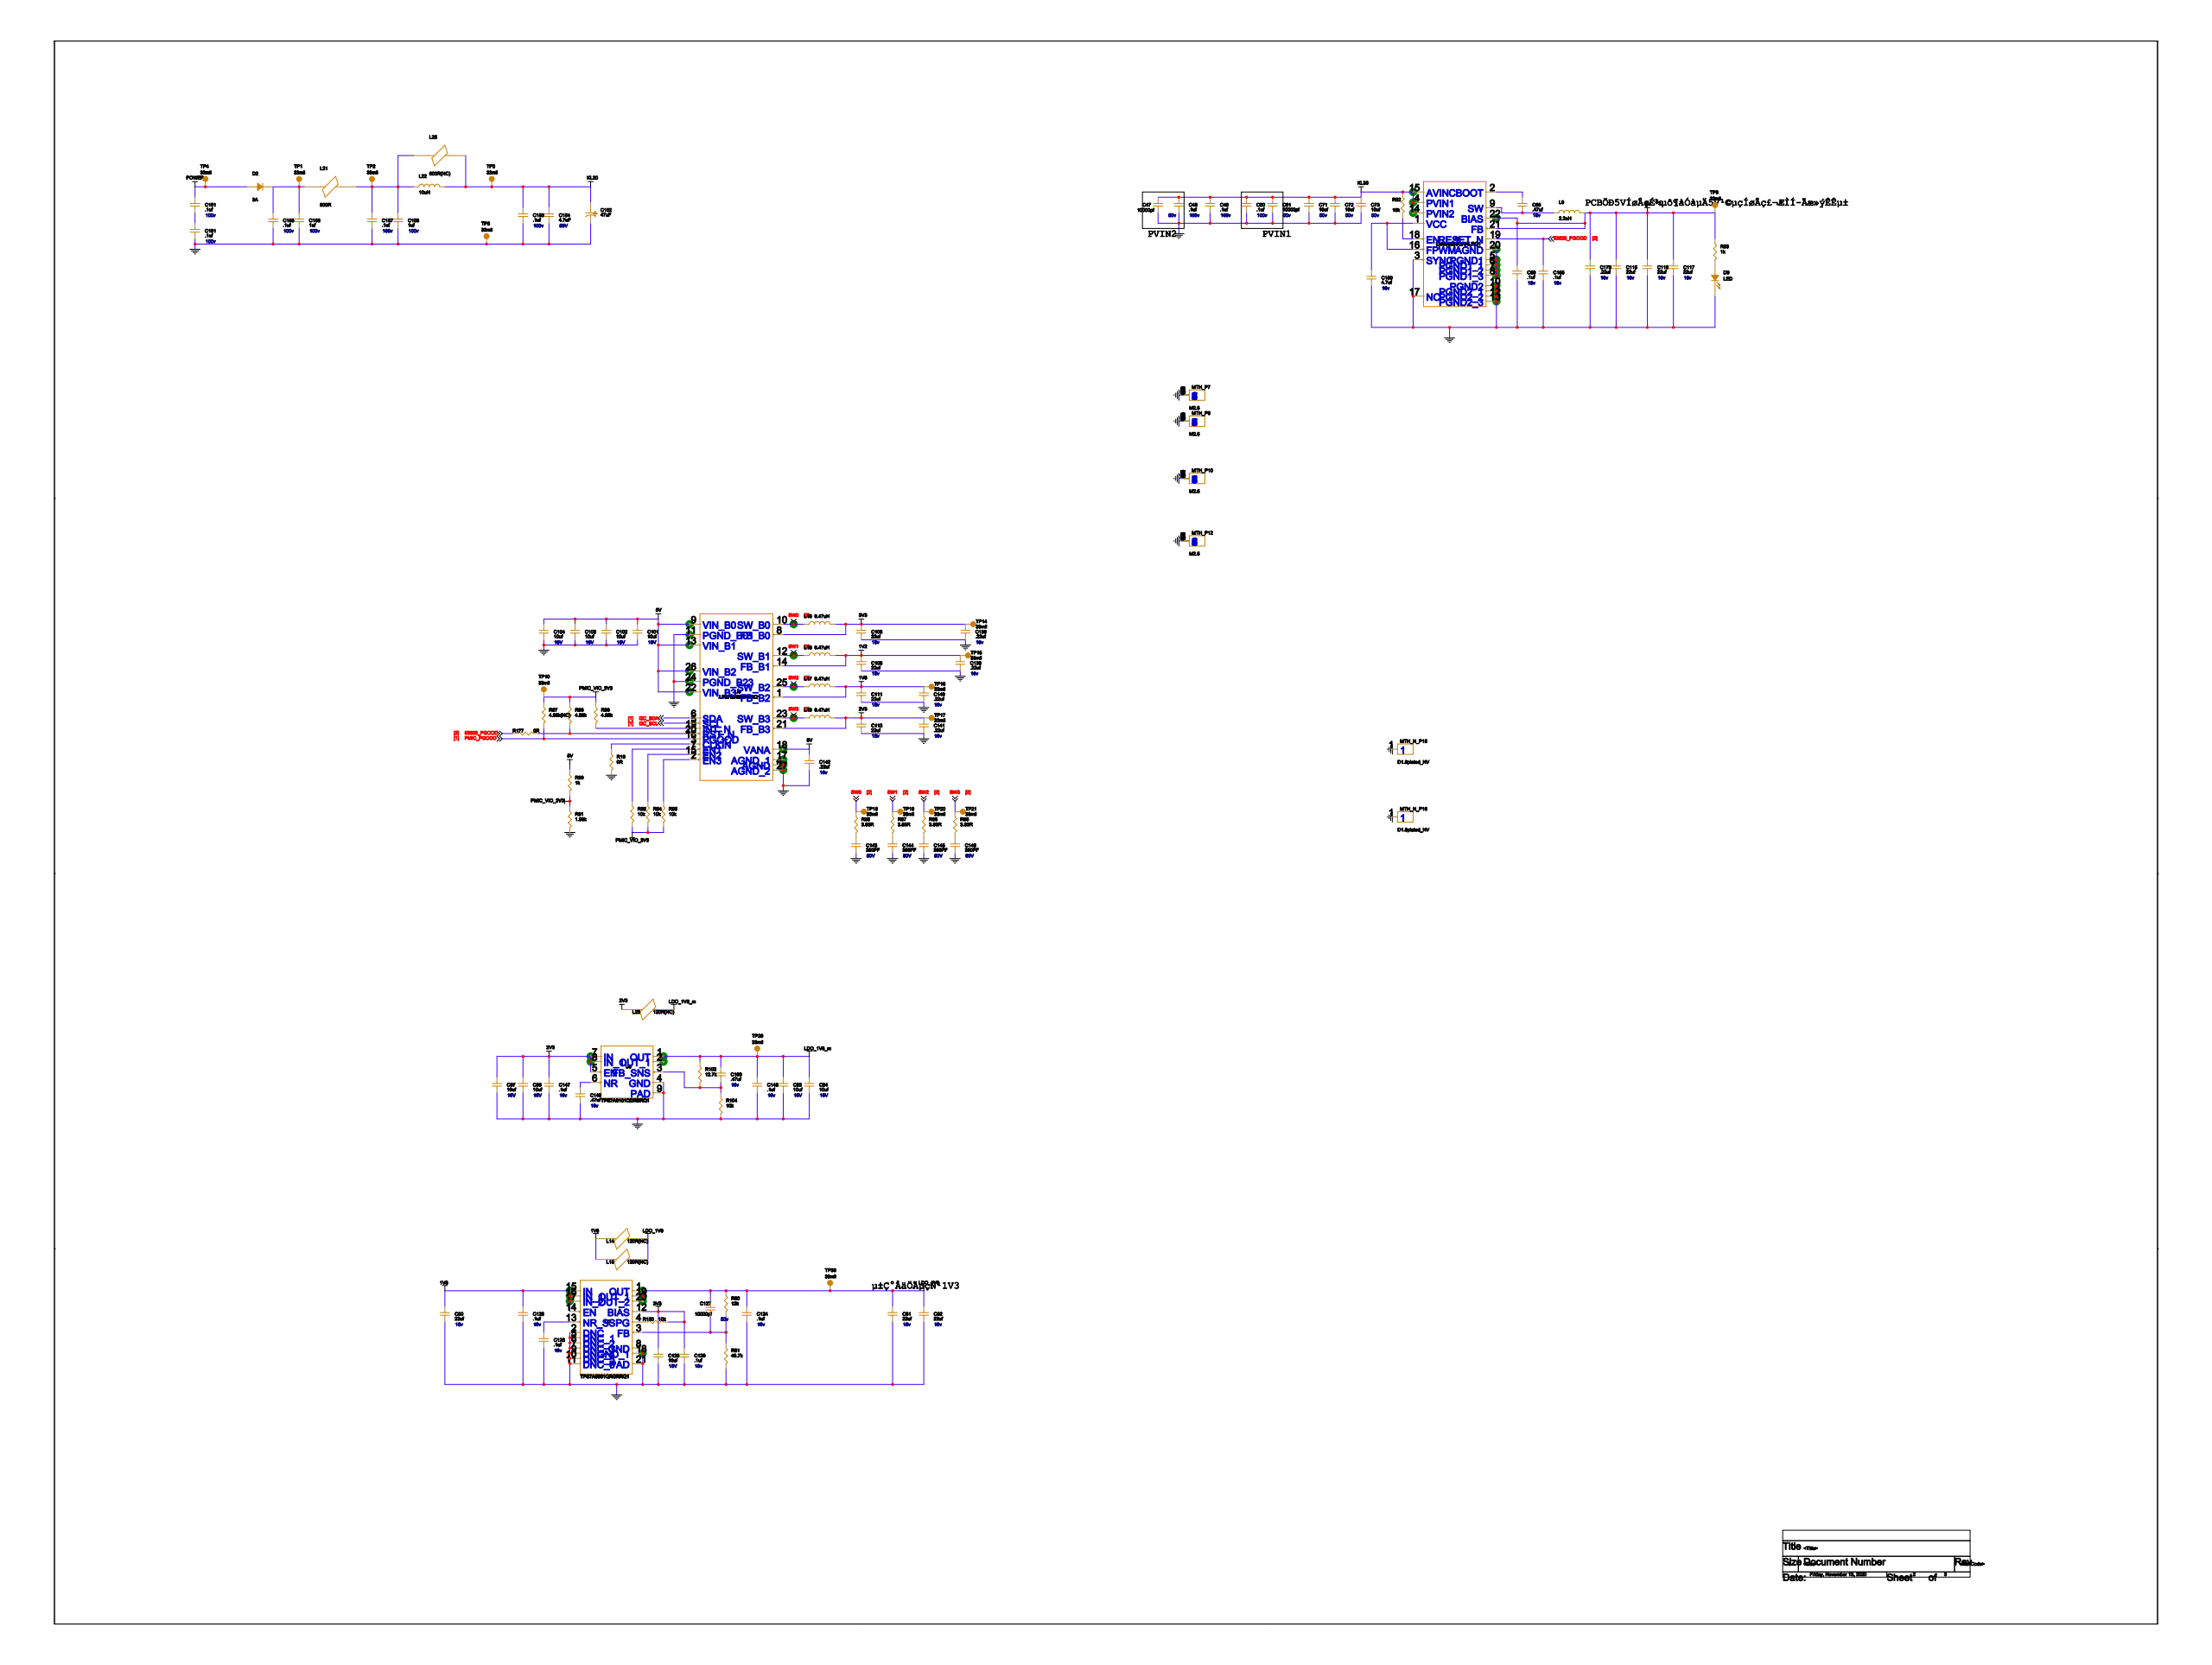Circuit board | Cadence Allegro | 338 parts | 150 nets | one sheet of the schematic
Parts on this sheet (reference | value | footprint):
C47 | 10000pf | C0402
C48 | .1uf | C0805
C49 | .1uf | C0805
C50 | .1uf | C0805
C51 | 10000pf | C0402
C55 | .47uf | C0603
C59 | .1uf | C0402
C71 | 10uf | C1210
C72 | 10uf | C1210
C73 | 10uf | C1210
C80 | 22uf | C1210
C81 | 22uf | C1210
C82 | 22uf | C1210
C83 | 10uf | C0805
C84 | 10uf | C0805
C86 | 10uf | C0805
C87 | 10uf | C0805
C101 | 10uf | C0805
C102 | 10uf | C0805
C103 | 10uf | C0805
C104 | 10uf | C0805
C105 | 22uf | C1210
C108 | 22uf | C1210
C111 | 22uf | C1210
C113 | 22uf | C1210
C115 | 22uf | C1210
C116 | 22uf | C1210
C117 | 22uf | C1210
C124 | .1uf | C0402
C125 | .1uf | C0402
C126 | .1uf | C0402
C127 | 10000pf | C0402
C128 | 10uf | C0805
C129 | .1uf | C0402
C138 | .22uf | C0402
C139 | .22uf | C0402
C140 | .22uf | C0402
C141 | .22uf | C0402
C142 | .22uf | C0402
C143 | 390PF | C0402
C144 | 390PF | C0402
C145 | 390PF | C0402
C146 | 390PF | C0402
C147 | .1uf | C0402
C148 | .1uf | C0402
C149 | .47uf | C0603
C151 | .1uf | C0805
C152 | 47uF | CAPAE630X800N
C153 | .1uf | C0805
C154 | 4.7uF | C0805
C155 | .1uf | C0805
C156 | 1uf | C0805
C157 | .1uf | C0805
C158 | 1uf | C0805
C161 | .1uf | C0805
C163 | .47uf | C0603
C179 | .22uf | C0402
C180 | 4.7uF | C0805
C185 | .1uf | C0402
D2 | 3A | SMB
D9 | LED | LED0603
L9 | 2.2uH | SPM5030
L14 | 120R(NC) | L0603
L15 | 120R(NC) | L0603
L16 | 0.47uH | L2520
L17 | 0.47uH | L2520
L18 | 0.47uH | L2520
L19 | 0.47uH | L2520
L21 | 600R | L0805
L22 | 10uH | SPM5030
L23 | 120R(NC) | L0603
L25 | 600R(NC) | L0805
MTH_N_P15 | D1.8plated_NV | MTGP240H180P
MTH_N_P16 | D1.8plated_NV | MTGP240H180P
MTH_P7 | M2.5 | MTGP600H290V6P
MTH_P8 | M2.5 | MTGP600H290V6P
MTH_P10 | M2.5 | MTGP600H290V6P
MTH_P12 | M2.5 | MTGP600H290V6P
R19 | 0R | R0402
R52 | 10k | R0402
R53 | 1k | R0603
R80 | 12k | R0402
R81 | 48.7k | R0402
R86 | 3.83R | R0402
R87 | 3.83R | R0402
R88 | 3.83R | R0402
R89 | 3.83R | R0402
R90 | 1k | R0402
R91 | 1.96k | R0402
R92 | 10k | R0402
R93 | 4.99k | R0402
R94 | 10k | R0402
R95 | 10k | R0402
R96 | 4.99k | R0402
R97 | 4.99k(NC) | R0402
R103 | 12.7k | R0402
R104 | 10k | R0402
R150 | 10k | R0402
R177 | 0R | R0402
TP1 | 33mil | TPAD_33MIL
TP2 | 33mil | TPAD_33MIL
TP3 | 33mil | TPAD_33MIL
TP4 | 33mil | TPAD_33MIL
TP6 | 33mil | TPAD_33MIL
TP9 | 33mil | TPAD_33MIL
TP10 | 33mil | TPAD_33MIL
TP14 | 33mil | TPAD_33MIL
TP15 | 33mil | TPAD_33MIL
TP16 | 33mil | TPAD_33MIL
TP17 | 33mil | TPAD_33MIL
TP18 | 33mil | TPAD_33MIL
TP19 | 33mil | TPAD_33MIL
TP20 | 33mil | TPAD_33MIL
TP21 | 33mil | TPAD_33MIL
TP29 | 33mil | TPAD_33MIL
TP30 | 33mil | TPAD_33MIL
U3 | LM536255QRNLRQ1 | RNL0022A
U5 | LP87524BRNFRQ1 | RNF0026C
U7 | TPS7A5301QRGRRQ1 | RGR0020A
U9 | TPS7A8101QDRBRQ1 | DRB0008A
Nets of these parts (net: part-pin ...):
N123549: C157-1 C158-1 L21-2 L22-1 L25-1 TP2-1
KL30: C47-1 C48-1 C49-1 C50-1 C51-1 C71-1 C72-1 C73-1 C152-1 C153-1 C154-1 L22-2 L25-2 R52-1 TP3-1 U3-4 U3-14 U3-15
POWER: C151-1 D2-2 TP4-1
PMIC_VIO_3V3: R90-2 R91-1 R92-2 R93-1 R94-2 R95-2 R96-1 R97-1 TP10-1
PMIC_PGOOD: R97-2 U5-16
GND: C47-2 C48-2 C49-2 C50-2 C51-2 C59-2 C71-2 C72-2 C73-2 C80-2 C81-2 C82-2 C83-2 C84-2 C86-2 C87-2 C101-2 C102-2 C103-2 C104-2 C105-2 C108-2 C111-2 C113-2 C115-2 C116-2 C117-2 C124-2 C125-2 C126-2 C128-2 C129-2 C138-2 C139-2 C140-2 C141-2 C142-2 C143-2 C144-2 C145-2 C146-2 C147-2 C148-2 C149-2 C152-2 C153-2 C154-2 C155-2 C156-2 C157-2 C158-2 C161-2 C179-2 C180-2 C185-2 D9-1 MTH_N_P15-1 MTH_N_P16-1 MTH_P7-1 MTH_P7-2 MTH_P7-3 MTH_P7-4 MTH_P7-5 MTH_P7-6 MTH_P7-7 MTH_P8-1 MTH_P8-2 MTH_P8-3 MTH_P8-4 MTH_P8-5 MTH_P8-6 MTH_P8-7 MTH_P10-1 MTH_P10-2 MTH_P10-3 MTH_P10-4 MTH_P10-5 MTH_P10-6 MTH_P10-7 MTH_P12-1 MTH_P12-2 MTH_P12-3 MTH_P12-4 MTH_P12-5 MTH_P12-6 MTH_P12-7 R19-2 R81-2 R91-2 R104-2 TP6-1 U9-4 U9-9 U3-3 U3-5 U3-6 U3-7 U3-8 U3-10 U3-11 U3-12 U3-13 U3-17 U3-20 U5-4 U5-11 U5-17 U5-24 U5-27 U7-2 U7-5 U7-6 U7-7 U7-8 U7-9 U7-10 U7-11 U7-18 U7-21
N78274: C127-2 R80-2 R81-1 U7-3
1V8: C80-1 C111-1 C125-1 C140-1 L14-1 L15-1 L17-2 TP16-1 U5-1 U7-14 U7-15 U7-16 U7-17
3V3: C105-1 C128-1 C129-1 C138-1 L16-2 R150-2 TP14-1 U5-8 U7-12
1V2: C108-1 C139-1 L18-2 TP15-1 U5-14
2V3: C86-1 C87-1 C113-1 C141-1 C147-1 L19-2 L23-1 TP17-1 U9-5 U9-7 U9-8 U5-21
5V: C59-1 C101-1 C102-1 C103-1 C104-1 C115-1 C116-1 C117-1 C142-1 C179-1 L9-2 R53-1 R90-1 TP9-1 U3-21 U3-22 U5-9 U5-13 U5-18 U5-22 U5-26
LDO_1V0: C81-1 C82-1 C124-1 C127-1 L14-2 L15-2 R80-1 TP30-1 U7-1 U7-19 U7-20
SW0: L16-1 R86-1 TP18-1 U5-10
N949950: C143-1 R86-2
SW1: L18-1 R87-1 TP19-1 U5-12
N957111: C144-1 R87-2
SW2: L17-1 R88-1 TP20-1 U5-25
N960781: C145-1 R88-2
SW3: L19-1 R89-1 TP21-1 U5-23
N964461: C146-1 R89-2
LDO_1V8_M: C83-1 C84-1 C148-1 C163-1 L23-2 R103-1 TP29-1 U9-1 U9-2
53625_PGOOD: C185-1 R177-1 U3-19
N77773: C126-1 U7-13
N123873: C151-2 C161-1
N123659: C155-1 C156-1 D2-1 L21-1 TP1-1
N39387: C180-1 U3-1 U3-16
N104639: C149-1 U9-6
N127180: C163-2 R103-2 R104-1 U9-3
N39067: C55-1 U3-2
N39291: C55-2 L9-1 U3-9
N394351: D9-2 R53-2
N39367: R52-2 U3-18
N516723: R150-1 U7-4
I2C_SDA: U5-6
I2C_SCL: U5-5
N98228: R92-1 U5-7
N98221: R94-1 U5-15
N98214: R95-1 U5-2
N598250: R96-2 R177-2 U5-20
N99204: R19-1 U5-3
N99352: R93-2 U5-19